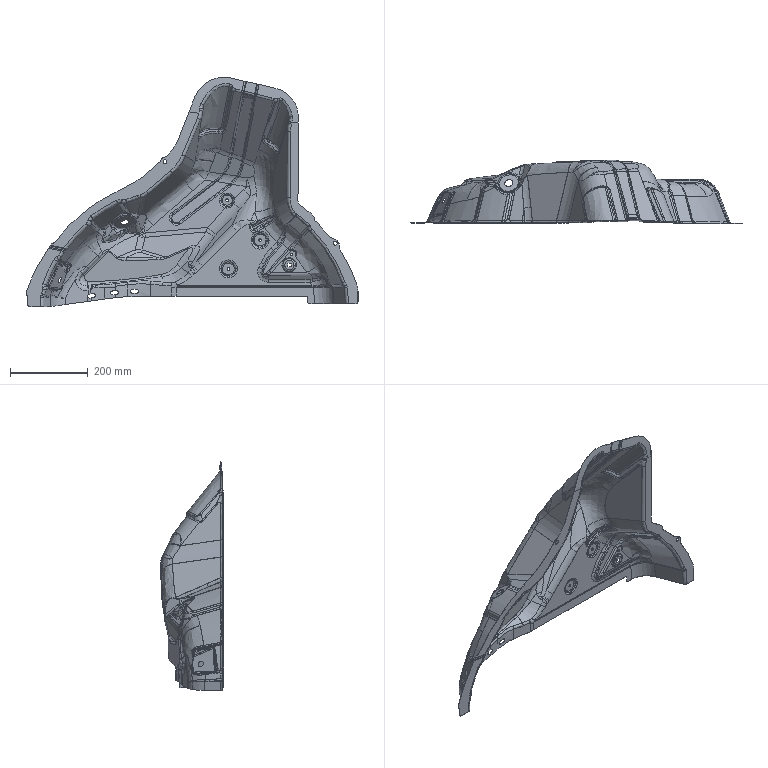Part | STEP file | FNA5401931 | 1 solid | 1342 faces | box 852.046 x 163.068 x 589.293 mm | volume 275736 mm3 | spline 1114 | cylinder 120 | plane 97 | other 11 | commonest cylinder face diameters 98.6 x8 100 x8 10 x7 6.5 x6 16 x6 17.4 x6